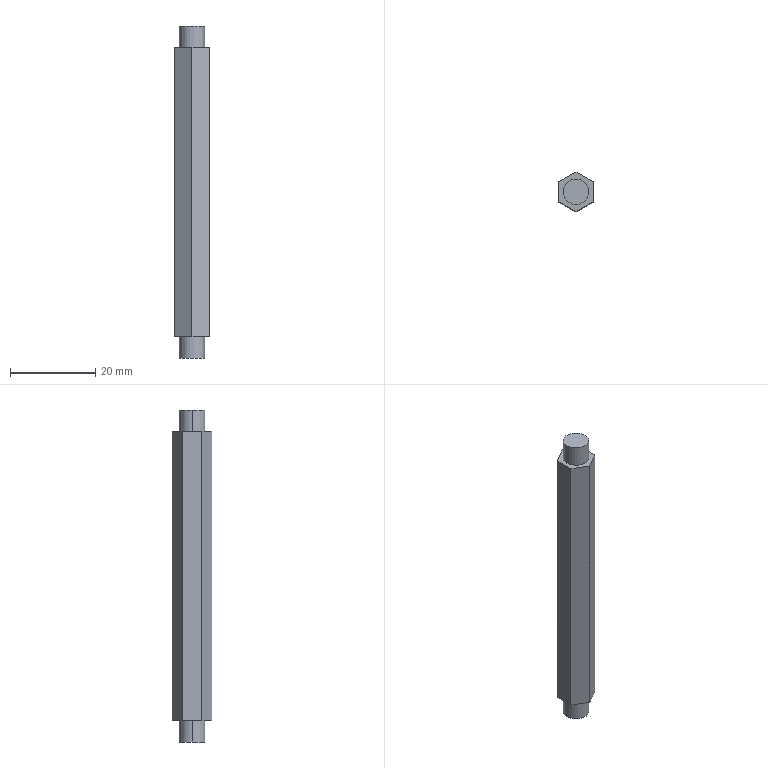Part | STEP file | 1 solid | 14 faces | box 8 x 9.238 x 78 mm | volume 4052 mm3 | plane 10 | cylinder 4 | commonest cylinder face diameters 6 x4
STEP:
#1=CARTESIAN_POINT('',(0.,0.,0.));
#2=DIRECTION('',(0.,0.,1.));
#3=DIRECTION('',(1.,0.,0.));
#4=AXIS2_PLACEMENT_3D('',#1,#2,#3);
#5=CARTESIAN_POINT('',(-5.42,-20.574,-52.535));
#6=VERTEX_POINT('',#5);
#7=CARTESIAN_POINT('',(-11.42,-20.574,-52.535));
#8=VERTEX_POINT('',#7);
#9=CARTESIAN_POINT('',(-8.42,-20.574,-52.535));
#10=DIRECTION('',(0.,0.,1.));
#11=DIRECTION('',(-1.,0.,0.));
#12=AXIS2_PLACEMENT_3D('',#9,#10,#11);
#13=CIRCLE('',#12,3.);
#14=CARTESIAN_POINT('',(-8.42,-20.574,-52.535));
#15=DIRECTION('',(0.,0.,-1.));
#16=DIRECTION('',(-1.,0.,0.));
#17=AXIS2_PLACEMENT_3D('',#14,#15,#16);
#18=CYLINDRICAL_SURFACE('',#17,3.);
#19=CARTESIAN_POINT('',(6.283,0.));
#20=DIRECTION('',(-1.,0.));
#21=VECTOR('',#20,1.);
#22=LINE('',#19,#21);
#23=(GEOMETRIC_REPRESENTATION_CONTEXT(2)PARAMETRIC_REPRESENTATION_CONTEXT()REPRESENTATION_CONTEXT('',''));
#24=DEFINITIONAL_REPRESENTATION('',(#22),#23);
#25=PCURVE('',#18,#24);
#26=CARTESIAN_POINT('',(-8.42,-20.574,-52.535));
#27=DIRECTION('',(0.,0.,-1.));
#28=DIRECTION('',(-1.,0.,0.));
#29=AXIS2_PLACEMENT_3D('',#26,#27,#28);
#30=PLANE('',#29);
#31=CARTESIAN_POINT('',(3.,0.));
#32=CARTESIAN_POINT('',(3.,-5.196));
#33=CARTESIAN_POINT('',(-1.5,-2.598));
#34=CARTESIAN_POINT('',(-6.,0.));
#35=CARTESIAN_POINT('',(-1.5,2.598));
#36=CARTESIAN_POINT('',(3.,5.196));
#37=CARTESIAN_POINT('',(3.,0.));
#38=(BOUNDED_CURVE()B_SPLINE_CURVE(2,(#31,#32,#33,#34,#35,#36,#37),.UNSPECIFIED.,.T.,.F.)B_SPLINE_CURVE_WITH_KNOTS((1,2,2,2,2,1),(-2.094,0.,2.094,4.189,6.283,8.378),.UNSPECIFIED.)CURVE()GEOMETRIC_REPRESENTATION_ITEM()RATIONAL_B_SPLINE_CURVE((1.,0.5,1.,0.5,1.,0.5,1.))REPRESENTATION_ITEM(''));
#39=(GEOMETRIC_REPRESENTATION_CONTEXT(2)PARAMETRIC_REPRESENTATION_CONTEXT()REPRESENTATION_CONTEXT('',''));
#40=DEFINITIONAL_REPRESENTATION('',(#38),#39);
#41=PCURVE('',#30,#40);
#42=SURFACE_CURVE('',#13,(#25,#41),.PCURVE_S1.);
#43=EDGE_CURVE('',#6,#8,#42,.T.);
#44=ORIENTED_EDGE('',*,*,#43,.F.);
#45=CARTESIAN_POINT('',(-5.42,-20.574,-57.535));
#46=VERTEX_POINT('',#45);
#47=CARTESIAN_POINT('',(-5.42,-20.574,-52.535));
#48=DIRECTION('',(0.,0.,-1.));
#49=VECTOR('',#48,1.);
#50=LINE('',#47,#49);
#51=CARTESIAN_POINT('',(3.142,0.));
#52=DIRECTION('',(0.,1.));
#53=VECTOR('',#52,1.);
#54=LINE('',#51,#53);
#55=(GEOMETRIC_REPRESENTATION_CONTEXT(2)PARAMETRIC_REPRESENTATION_CONTEXT()REPRESENTATION_CONTEXT('',''));
#56=DEFINITIONAL_REPRESENTATION('',(#54),#55);
#57=PCURVE('',#18,#56);
#58=CARTESIAN_POINT('',(-8.42,-20.574,-52.535));
#59=DIRECTION('',(0.,0.,-1.));
#60=DIRECTION('',(-1.,0.,0.));
#61=AXIS2_PLACEMENT_3D('',#58,#59,#60);
#62=CYLINDRICAL_SURFACE('',#61,3.);
#63=CARTESIAN_POINT('',(3.142,0.));
#64=DIRECTION('',(0.,1.));
#65=VECTOR('',#64,1.);
#66=LINE('',#63,#65);
#67=(GEOMETRIC_REPRESENTATION_CONTEXT(2)PARAMETRIC_REPRESENTATION_CONTEXT()REPRESENTATION_CONTEXT('',''));
#68=DEFINITIONAL_REPRESENTATION('',(#66),#67);
#69=PCURVE('',#62,#68);
#70=SURFACE_CURVE('',#50,(#57,#69),.PCURVE_S1.);
#71=EDGE_CURVE('',#6,#46,#70,.T.);
#72=ORIENTED_EDGE('',*,*,#71,.T.);
#73=CARTESIAN_POINT('',(-11.42,-20.574,-57.535));
#74=VERTEX_POINT('',#73);
#75=CARTESIAN_POINT('',(-8.42,-20.574,-57.535));
#76=DIRECTION('',(0.,0.,1.));
#77=DIRECTION('',(-1.,0.,0.));
#78=AXIS2_PLACEMENT_3D('',#75,#76,#77);
#79=CIRCLE('',#78,3.);
#80=CARTESIAN_POINT('',(6.283,5.));
#81=DIRECTION('',(-1.,0.));
#82=VECTOR('',#81,1.);
#83=LINE('',#80,#82);
#84=(GEOMETRIC_REPRESENTATION_CONTEXT(2)PARAMETRIC_REPRESENTATION_CONTEXT()REPRESENTATION_CONTEXT('',''));
#85=DEFINITIONAL_REPRESENTATION('',(#83),#84);
#86=PCURVE('',#18,#85);
#87=CARTESIAN_POINT('',(-8.42,-20.574,-57.535));
#88=DIRECTION('',(0.,0.,1.));
#89=DIRECTION('',(1.,0.,0.));
#90=AXIS2_PLACEMENT_3D('',#87,#88,#89);
#91=PLANE('',#90);
#92=CARTESIAN_POINT('',(0.,0.));
#93=DIRECTION('',(-1.,0.));
#94=AXIS2_PLACEMENT_2D('',#92,#93);
#95=CIRCLE('',#94,3.);
#96=(GEOMETRIC_REPRESENTATION_CONTEXT(2)PARAMETRIC_REPRESENTATION_CONTEXT()REPRESENTATION_CONTEXT('',''));
#97=DEFINITIONAL_REPRESENTATION('',(#95),#96);
#98=PCURVE('',#91,#97);
#99=SURFACE_CURVE('',#79,(#86,#98),.PCURVE_S1.);
#100=EDGE_CURVE('',#46,#74,#99,.T.);
#101=ORIENTED_EDGE('',*,*,#100,.T.);
#102=CARTESIAN_POINT('',(-11.42,-20.574,-52.535));
#103=DIRECTION('',(0.,0.,-1.));
#104=VECTOR('',#103,1.);
#105=LINE('',#102,#104);
#106=CARTESIAN_POINT('',(0.,0.));
#107=DIRECTION('',(0.,1.));
#108=VECTOR('',#107,1.);
#109=LINE('',#106,#108);
#110=(GEOMETRIC_REPRESENTATION_CONTEXT(2)PARAMETRIC_REPRESENTATION_CONTEXT()REPRESENTATION_CONTEXT('',''));
#111=DEFINITIONAL_REPRESENTATION('',(#109),#110);
#112=PCURVE('',#18,#111);
#113=CARTESIAN_POINT('',(6.283,0.));
#114=DIRECTION('',(0.,1.));
#115=VECTOR('',#114,1.);
#116=LINE('',#113,#115);
#117=(GEOMETRIC_REPRESENTATION_CONTEXT(2)PARAMETRIC_REPRESENTATION_CONTEXT()REPRESENTATION_CONTEXT('',''));
#118=DEFINITIONAL_REPRESENTATION('',(#116),#117);
#119=PCURVE('',#62,#118);
#120=SURFACE_CURVE('',#105,(#112,#119),.PCURVE_S1.);
#121=EDGE_CURVE('',#8,#74,#120,.T.);
#122=ORIENTED_EDGE('',*,*,#121,.F.);
#123=EDGE_LOOP('',(#44,#72,#101,#122));
#124=FACE_BOUND('',#123,.T.);
#125=ADVANCED_FACE('',(#124),#18,.T.);
#126=CARTESIAN_POINT('',(-11.42,-20.574,20.465));
#127=VERTEX_POINT('',#126);
#128=CARTESIAN_POINT('',(-5.42,-20.574,20.465));
#129=VERTEX_POINT('',#128);
#130=CARTESIAN_POINT('',(-8.42,-20.574,20.465));
#131=DIRECTION('',(0.,0.,-1.));
#132=DIRECTION('',(-1.,0.,0.));
#133=AXIS2_PLACEMENT_3D('',#130,#131,#132);
#134=CIRCLE('',#133,3.);
#135=CARTESIAN_POINT('',(-8.42,-20.574,15.465));
#136=DIRECTION('',(0.,0.,-1.));
#137=DIRECTION('',(-1.,0.,0.));
#138=AXIS2_PLACEMENT_3D('',#135,#136,#137);
#139=CYLINDRICAL_SURFACE('',#138,3.);
#140=CARTESIAN_POINT('',(0.,-5.));
#141=DIRECTION('',(1.,0.));
#142=VECTOR('',#141,1.);
#143=LINE('',#140,#142);
#144=(GEOMETRIC_REPRESENTATION_CONTEXT(2)PARAMETRIC_REPRESENTATION_CONTEXT()REPRESENTATION_CONTEXT('',''));
#145=DEFINITIONAL_REPRESENTATION('',(#143),#144);
#146=PCURVE('',#139,#145);
#147=CARTESIAN_POINT('',(-8.42,-20.574,20.465));
#148=DIRECTION('',(0.,0.,1.));
#149=DIRECTION('',(1.,0.,0.));
#150=AXIS2_PLACEMENT_3D('',#147,#148,#149);
#151=PLANE('',#150);
#152=CARTESIAN_POINT('',(-3.,0.));
#153=CARTESIAN_POINT('',(-3.,5.196));
#154=CARTESIAN_POINT('',(1.5,2.598));
#155=CARTESIAN_POINT('',(6.,0.));
#156=CARTESIAN_POINT('',(1.5,-2.598));
#157=CARTESIAN_POINT('',(-3.,-5.196));
#158=CARTESIAN_POINT('',(-3.,0.));
#159=(BOUNDED_CURVE()B_SPLINE_CURVE(2,(#152,#153,#154,#155,#156,#157,#158),.UNSPECIFIED.,.T.,.F.)B_SPLINE_CURVE_WITH_KNOTS((1,2,2,2,2,1),(-2.094,0.,2.094,4.189,6.283,8.378),.UNSPECIFIED.)CURVE()GEOMETRIC_REPRESENTATION_ITEM()RATIONAL_B_SPLINE_CURVE((1.,0.5,1.,0.5,1.,0.5,1.))REPRESENTATION_ITEM(''));
#160=(GEOMETRIC_REPRESENTATION_CONTEXT(2)PARAMETRIC_REPRESENTATION_CONTEXT()REPRESENTATION_CONTEXT('',''));
#161=DEFINITIONAL_REPRESENTATION('',(#159),#160);
#162=PCURVE('',#151,#161);
#163=SURFACE_CURVE('',#134,(#146,#162),.PCURVE_S1.);
#164=EDGE_CURVE('',#127,#129,#163,.T.);
#165=ORIENTED_EDGE('',*,*,#164,.T.);
#166=CARTESIAN_POINT('',(-5.42,-20.574,15.465));
#167=VERTEX_POINT('',#166);
#168=CARTESIAN_POINT('',(-5.42,-20.574,15.465));
#169=DIRECTION('',(0.,0.,-1.));
#170=VECTOR('',#169,1.);
#171=LINE('',#168,#170);
#172=CARTESIAN_POINT('',(3.142,0.));
#173=DIRECTION('',(0.,1.));
#174=VECTOR('',#173,1.);
#175=LINE('',#172,#174);
#176=(GEOMETRIC_REPRESENTATION_CONTEXT(2)PARAMETRIC_REPRESENTATION_CONTEXT()REPRESENTATION_CONTEXT('',''));
#177=DEFINITIONAL_REPRESENTATION('',(#175),#176);
#178=PCURVE('',#139,#177);
#179=CARTESIAN_POINT('',(-8.42,-20.574,15.465));
#180=DIRECTION('',(0.,0.,-1.));
#181=DIRECTION('',(-1.,0.,0.));
#182=AXIS2_PLACEMENT_3D('',#179,#180,#181);
#183=CYLINDRICAL_SURFACE('',#182,3.);
#184=CARTESIAN_POINT('',(3.142,0.));
#185=DIRECTION('',(0.,1.));
#186=VECTOR('',#185,1.);
#187=LINE('',#184,#186);
#188=(GEOMETRIC_REPRESENTATION_CONTEXT(2)PARAMETRIC_REPRESENTATION_CONTEXT()REPRESENTATION_CONTEXT('',''));
#189=DEFINITIONAL_REPRESENTATION('',(#187),#188);
#190=PCURVE('',#183,#189);
#191=SURFACE_CURVE('',#171,(#178,#190),.PCURVE_S1.);
#192=EDGE_CURVE('',#129,#167,#191,.T.);
#193=ORIENTED_EDGE('',*,*,#192,.T.);
#194=CARTESIAN_POINT('',(-11.42,-20.574,15.465));
#195=VERTEX_POINT('',#194);
#196=CARTESIAN_POINT('',(-8.42,-20.574,15.465));
#197=DIRECTION('',(0.,0.,-1.));
#198=DIRECTION('',(-1.,0.,0.));
#199=AXIS2_PLACEMENT_3D('',#196,#197,#198);
#200=CIRCLE('',#199,3.);
#201=CARTESIAN_POINT('',(0.,0.));
#202=DIRECTION('',(1.,0.));
#203=VECTOR('',#202,1.);
#204=LINE('',#201,#203);
#205=(GEOMETRIC_REPRESENTATION_CONTEXT(2)PARAMETRIC_REPRESENTATION_CONTEXT()REPRESENTATION_CONTEXT('',''));
#206=DEFINITIONAL_REPRESENTATION('',(#204),#205);
#207=PCURVE('',#139,#206);
#208=CARTESIAN_POINT('',(-8.42,-20.574,15.465));
#209=DIRECTION('',(0.,0.,1.));
#210=DIRECTION('',(1.,0.,0.));
#211=AXIS2_PLACEMENT_3D('',#208,#209,#210);
#212=PLANE('',#211);
#213=CARTESIAN_POINT('',(-3.,0.));
#214=CARTESIAN_POINT('',(-3.,5.196));
#215=CARTESIAN_POINT('',(1.5,2.598));
#216=CARTESIAN_POINT('',(6.,0.));
#217=CARTESIAN_POINT('',(1.5,-2.598));
#218=CARTESIAN_POINT('',(-3.,-5.196));
#219=CARTESIAN_POINT('',(-3.,0.));
#220=(BOUNDED_CURVE()B_SPLINE_CURVE(2,(#213,#214,#215,#216,#217,#218,#219),.UNSPECIFIED.,.T.,.F.)B_SPLINE_CURVE_WITH_KNOTS((1,2,2,2,2,1),(-2.094,0.,2.094,4.189,6.283,8.378),.UNSPECIFIED.)CURVE()GEOMETRIC_REPRESENTATION_ITEM()RATIONAL_B_SPLINE_CURVE((1.,0.5,1.,0.5,1.,0.5,1.))REPRESENTATION_ITEM(''));
#221=(GEOMETRIC_REPRESENTATION_CONTEXT(2)PARAMETRIC_REPRESENTATION_CONTEXT()REPRESENTATION_CONTEXT('',''));
#222=DEFINITIONAL_REPRESENTATION('',(#220),#221);
#223=PCURVE('',#212,#222);
#224=SURFACE_CURVE('',#200,(#207,#223),.PCURVE_S1.);
#225=EDGE_CURVE('',#195,#167,#224,.T.);
#226=ORIENTED_EDGE('',*,*,#225,.F.);
#227=CARTESIAN_POINT('',(-11.42,-20.574,15.465));
#228=DIRECTION('',(0.,0.,-1.));
#229=VECTOR('',#228,1.);
#230=LINE('',#227,#229);
#231=CARTESIAN_POINT('',(0.,0.));
#232=DIRECTION('',(0.,1.));
#233=VECTOR('',#232,1.);
#234=LINE('',#231,#233);
#235=(GEOMETRIC_REPRESENTATION_CONTEXT(2)PARAMETRIC_REPRESENTATION_CONTEXT()REPRESENTATION_CONTEXT('',''));
#236=DEFINITIONAL_REPRESENTATION('',(#234),#235);
#237=PCURVE('',#139,#236);
#238=CARTESIAN_POINT('',(6.283,0.));
#239=DIRECTION('',(0.,1.));
#240=VECTOR('',#239,1.);
#241=LINE('',#238,#240);
#242=(GEOMETRIC_REPRESENTATION_CONTEXT(2)PARAMETRIC_REPRESENTATION_CONTEXT()REPRESENTATION_CONTEXT('',''));
#243=DEFINITIONAL_REPRESENTATION('',(#241),#242);
#244=PCURVE('',#183,#243);
#245=SURFACE_CURVE('',#230,(#237,#244),.PCURVE_S1.);
#246=EDGE_CURVE('',#127,#195,#245,.T.);
#247=ORIENTED_EDGE('',*,*,#246,.F.);
#248=EDGE_LOOP('',(#165,#193,#226,#247));
#249=FACE_BOUND('',#248,.T.);
#250=ADVANCED_FACE('',(#249),#139,.T.);
#251=CARTESIAN_POINT('',(-8.42,-25.193,15.465));
#252=VERTEX_POINT('',#251);
#253=CARTESIAN_POINT('',(-8.42,-25.193,-52.535));
#254=VERTEX_POINT('',#253);
#255=CARTESIAN_POINT('',(-8.42,-25.193,-18.535));
#256=DIRECTION('',(0.,0.,-1.));
#257=VECTOR('',#256,1.);
#258=LINE('',#255,#257);
#259=CARTESIAN_POINT('',(-8.42,-25.193,-18.535));
#260=DIRECTION('',(0.5,-0.866,0.));
#261=DIRECTION('',(0.866,0.5,0.));
#262=AXIS2_PLACEMENT_3D('',#259,#260,#261);
#263=PLANE('',#262);
#264=CARTESIAN_POINT('',(0.,0.));
#265=DIRECTION('',(0.,-1.));
#266=VECTOR('',#265,1.);
#267=LINE('',#264,#266);
#268=(GEOMETRIC_REPRESENTATION_CONTEXT(2)PARAMETRIC_REPRESENTATION_CONTEXT()REPRESENTATION_CONTEXT('',''));
#269=DEFINITIONAL_REPRESENTATION('',(#267),#268);
#270=PCURVE('',#263,#269);
#271=CARTESIAN_POINT('',(-12.42,-22.883,-18.535));
#272=DIRECTION('',(-0.5,-0.866,0.));
#273=DIRECTION('',(0.866,-0.5,0.));
#274=AXIS2_PLACEMENT_3D('',#271,#272,#273);
#275=PLANE('',#274);
#276=CARTESIAN_POINT('',(4.619,0.));
#277=DIRECTION('',(0.,-1.));
#278=VECTOR('',#277,1.);
#279=LINE('',#276,#278);
#280=(GEOMETRIC_REPRESENTATION_CONTEXT(2)PARAMETRIC_REPRESENTATION_CONTEXT()REPRESENTATION_CONTEXT('',''));
#281=DEFINITIONAL_REPRESENTATION('',(#279),#280);
#282=PCURVE('',#275,#281);
#283=SURFACE_CURVE('',#258,(#270,#282),.PCURVE_S1.);
#284=EDGE_CURVE('',#252,#254,#283,.T.);
#285=ORIENTED_EDGE('',*,*,#284,.T.);
#286=CARTESIAN_POINT('',(-4.42,-22.883,-52.535));
#287=VERTEX_POINT('',#286);
#288=CARTESIAN_POINT('',(-8.42,-25.193,-52.535));
#289=DIRECTION('',(0.866,0.5,0.));
#290=VECTOR('',#289,1.);
#291=LINE('',#288,#290);
#292=CARTESIAN_POINT('',(0.,-34.));
#293=DIRECTION('',(1.,0.));
#294=VECTOR('',#293,1.);
#295=LINE('',#292,#294);
#296=(GEOMETRIC_REPRESENTATION_CONTEXT(2)PARAMETRIC_REPRESENTATION_CONTEXT()REPRESENTATION_CONTEXT('',''));
#297=DEFINITIONAL_REPRESENTATION('',(#295),#296);
#298=PCURVE('',#263,#297);
#299=CARTESIAN_POINT('',(0.,-4.619));
#300=DIRECTION('',(-0.866,0.5));
#301=VECTOR('',#300,1.);
#302=LINE('',#299,#301);
#303=(GEOMETRIC_REPRESENTATION_CONTEXT(2)PARAMETRIC_REPRESENTATION_CONTEXT()REPRESENTATION_CONTEXT('',''));
#304=DEFINITIONAL_REPRESENTATION('',(#302),#303);
#305=PCURVE('',#30,#304);
#306=SURFACE_CURVE('',#291,(#298,#305),.PCURVE_S1.);
#307=EDGE_CURVE('',#254,#287,#306,.T.);
#308=ORIENTED_EDGE('',*,*,#307,.T.);
#309=CARTESIAN_POINT('',(-4.42,-22.883,15.465));
#310=VERTEX_POINT('',#309);
#311=CARTESIAN_POINT('',(-4.42,-22.883,-18.535));
#312=DIRECTION('',(0.,0.,1.));
#313=VECTOR('',#312,1.);
#314=LINE('',#311,#313);
#315=CARTESIAN_POINT('',(4.619,0.));
#316=DIRECTION('',(0.,1.));
#317=VECTOR('',#316,1.);
#318=LINE('',#315,#317);
#319=(GEOMETRIC_REPRESENTATION_CONTEXT(2)PARAMETRIC_REPRESENTATION_CONTEXT()REPRESENTATION_CONTEXT('',''));
#320=DEFINITIONAL_REPRESENTATION('',(#318),#319);
#321=PCURVE('',#263,#320);
#322=CARTESIAN_POINT('',(-4.42,-22.883,-18.535));
#323=DIRECTION('',(1.,0.,0.));
#324=DIRECTION('',(0.,1.,0.));
#325=AXIS2_PLACEMENT_3D('',#322,#323,#324);
#326=PLANE('',#325);
#327=CARTESIAN_POINT('',(0.,0.));
#328=DIRECTION('',(0.,1.));
#329=VECTOR('',#328,1.);
#330=LINE('',#327,#329);
#331=(GEOMETRIC_REPRESENTATION_CONTEXT(2)PARAMETRIC_REPRESENTATION_CONTEXT()REPRESENTATION_CONTEXT('',''));
#332=DEFINITIONAL_REPRESENTATION('',(#330),#331);
#333=PCURVE('',#326,#332);
#334=SURFACE_CURVE('',#314,(#321,#333),.PCURVE_S1.);
#335=EDGE_CURVE('',#287,#310,#334,.T.);
#336=ORIENTED_EDGE('',*,*,#335,.T.);
#337=CARTESIAN_POINT('',(-8.42,-25.193,15.465));
#338=DIRECTION('',(-0.866,-0.5,0.));
#339=VECTOR('',#338,1.);
#340=LINE('',#337,#339);
#341=CARTESIAN_POINT('',(0.,34.));
#342=DIRECTION('',(-1.,0.));
#343=VECTOR('',#342,1.);
#344=LINE('',#341,#343);
#345=(GEOMETRIC_REPRESENTATION_CONTEXT(2)PARAMETRIC_REPRESENTATION_CONTEXT()REPRESENTATION_CONTEXT('',''));
#346=DEFINITIONAL_REPRESENTATION('',(#344),#345);
#347=PCURVE('',#263,#346);
#348=CARTESIAN_POINT('',(0.,-4.619));
#349=DIRECTION('',(-0.866,-0.5));
#350=VECTOR('',#349,1.);
#351=LINE('',#348,#350);
#352=(GEOMETRIC_REPRESENTATION_CONTEXT(2)PARAMETRIC_REPRESENTATION_CONTEXT()REPRESENTATION_CONTEXT('',''));
#353=DEFINITIONAL_REPRESENTATION('',(#351),#352);
#354=PCURVE('',#212,#353);
#355=SURFACE_CURVE('',#340,(#347,#354),.PCURVE_S1.);
#356=EDGE_CURVE('',#310,#252,#355,.T.);
#357=ORIENTED_EDGE('',*,*,#356,.T.);
#358=EDGE_LOOP('',(#285,#308,#336,#357));
#359=FACE_BOUND('',#358,.T.);
#360=ADVANCED_FACE('',(#359),#263,.T.);
#361=CARTESIAN_POINT('',(-12.42,-22.883,-52.535));
#362=VERTEX_POINT('',#361);
#363=CARTESIAN_POINT('',(-8.42,-25.193,-52.535));
#364=DIRECTION('',(-0.866,0.5,0.));
#365=VECTOR('',#364,1.);
#366=LINE('',#363,#365);
#367=CARTESIAN_POINT('',(0.,-4.619));
#368=DIRECTION('',(0.866,0.5));
#369=VECTOR('',#368,1.);
#370=LINE('',#367,#369);
#371=(GEOMETRIC_REPRESENTATION_CONTEXT(2)PARAMETRIC_REPRESENTATION_CONTEXT()REPRESENTATION_CONTEXT('',''));
#372=DEFINITIONAL_REPRESENTATION('',(#370),#371);
#373=PCURVE('',#30,#372);
#374=CARTESIAN_POINT('',(4.619,-34.));
#375=DIRECTION('',(-1.,0.));
#376=VECTOR('',#375,1.);
#377=LINE('',#374,#376);
#378=(GEOMETRIC_REPRESENTATION_CONTEXT(2)PARAMETRIC_REPRESENTATION_CONTEXT()REPRESENTATION_CONTEXT('',''));
#379=DEFINITIONAL_REPRESENTATION('',(#377),#378);
#380=PCURVE('',#275,#379);
#381=SURFACE_CURVE('',#366,(#373,#380),.PCURVE_S1.);
#382=EDGE_CURVE('',#254,#362,#381,.T.);
#383=ORIENTED_EDGE('',*,*,#382,.T.);
#384=CARTESIAN_POINT('',(-12.42,-18.264,-52.535));
#385=VERTEX_POINT('',#384);
#386=CARTESIAN_POINT('',(-12.42,-20.574,-52.535));
#387=DIRECTION('',(0.,1.,0.));
#388=VECTOR('',#387,1.);
#389=LINE('',#386,#388);
#390=CARTESIAN_POINT('',(4.,0.));
#391=DIRECTION('',(0.,1.));
#392=VECTOR('',#391,1.);
#393=LINE('',#390,#392);
#394=(GEOMETRIC_REPRESENTATION_CONTEXT(2)PARAMETRIC_REPRESENTATION_CONTEXT()REPRESENTATION_CONTEXT('',''));
#395=DEFINITIONAL_REPRESENTATION('',(#393),#394);
#396=PCURVE('',#30,#395);
#397=CARTESIAN_POINT('',(-12.42,-18.264,-18.535));
#398=DIRECTION('',(-1.,0.,0.));
#399=DIRECTION('',(0.,-1.,0.));
#400=AXIS2_PLACEMENT_3D('',#397,#398,#399);
#401=PLANE('',#400);
#402=CARTESIAN_POINT('',(2.309,-34.));
#403=DIRECTION('',(-1.,0.));
#404=VECTOR('',#403,1.);
#405=LINE('',#402,#404);
#406=(GEOMETRIC_REPRESENTATION_CONTEXT(2)PARAMETRIC_REPRESENTATION_CONTEXT()REPRESENTATION_CONTEXT('',''));
#407=DEFINITIONAL_REPRESENTATION('',(#405),#406);
#408=PCURVE('',#401,#407);
#409=SURFACE_CURVE('',#389,(#396,#408),.PCURVE_S1.);
#410=EDGE_CURVE('',#362,#385,#409,.T.);
#411=ORIENTED_EDGE('',*,*,#410,.T.);
#412=CARTESIAN_POINT('',(-8.42,-15.955,-52.535));
#413=VERTEX_POINT('',#412);
#414=CARTESIAN_POINT('',(-12.42,-18.264,-52.535));
#415=DIRECTION('',(0.866,0.5,0.));
#416=VECTOR('',#415,1.);
#417=LINE('',#414,#416);
#418=CARTESIAN_POINT('',(4.,2.309));
#419=DIRECTION('',(-0.866,0.5));
#420=VECTOR('',#419,1.);
#421=LINE('',#418,#420);
#422=(GEOMETRIC_REPRESENTATION_CONTEXT(2)PARAMETRIC_REPRESENTATION_CONTEXT()REPRESENTATION_CONTEXT('',''));
#423=DEFINITIONAL_REPRESENTATION('',(#421),#422);
#424=PCURVE('',#30,#423);
#425=CARTESIAN_POINT('',(-8.42,-15.955,-18.535));
#426=DIRECTION('',(-0.5,0.866,0.));
#427=DIRECTION('',(-0.866,-0.5,0.));
#428=AXIS2_PLACEMENT_3D('',#425,#426,#427);
#429=PLANE('',#428);
#430=CARTESIAN_POINT('',(4.619,-34.));
#431=DIRECTION('',(-1.,0.));
#432=VECTOR('',#431,1.);
#433=LINE('',#430,#432);
#434=(GEOMETRIC_REPRESENTATION_CONTEXT(2)PARAMETRIC_REPRESENTATION_CONTEXT()REPRESENTATION_CONTEXT('',''));
#435=DEFINITIONAL_REPRESENTATION('',(#433),#434);
#436=PCURVE('',#429,#435);
#437=SURFACE_CURVE('',#417,(#424,#436),.PCURVE_S1.);
#438=EDGE_CURVE('',#385,#413,#437,.T.);
#439=ORIENTED_EDGE('',*,*,#438,.T.);
#440=CARTESIAN_POINT('',(-4.42,-18.264,-52.535));
#441=VERTEX_POINT('',#440);
#442=CARTESIAN_POINT('',(-8.42,-15.955,-52.535));
#443=DIRECTION('',(0.866,-0.5,0.));
#444=VECTOR('',#443,1.);
#445=LINE('',#442,#444);
#446=CARTESIAN_POINT('',(0.,4.619));
#447=DIRECTION('',(-0.866,-0.5));
#448=VECTOR('',#447,1.);
#449=LINE('',#446,#448);
#450=(GEOMETRIC_REPRESENTATION_CONTEXT(2)PARAMETRIC_REPRESENTATION_CONTEXT()REPRESENTATION_CONTEXT('',''));
#451=DEFINITIONAL_REPRESENTATION('',(#449),#450);
#452=PCURVE('',#30,#451);
#453=CARTESIAN_POINT('',(-4.42,-18.264,-18.535));
#454=DIRECTION('',(0.5,0.866,0.));
#455=DIRECTION('',(-0.866,0.5,0.));
#456=AXIS2_PLACEMENT_3D('',#453,#454,#455);
#457=PLANE('',#456);
#458=CARTESIAN_POINT('',(4.619,-34.));
#459=DIRECTION('',(-1.,0.));
#460=VECTOR('',#459,1.);
#461=LINE('',#458,#460);
#462=(GEOMETRIC_REPRESENTATION_CONTEXT(2)PARAMETRIC_REPRESENTATION_CONTEXT()REPRESENTATION_CONTEXT('',''));
#463=DEFINITIONAL_REPRESENTATION('',(#461),#462);
#464=PCURVE('',#457,#463);
#465=SURFACE_CURVE('',#445,(#452,#464),.PCURVE_S1.);
#466=EDGE_CURVE('',#413,#441,#465,.T.);
#467=ORIENTED_EDGE('',*,*,#466,.T.);
#468=CARTESIAN_POINT('',(-4.42,-20.574,-52.535));
#469=DIRECTION('',(0.,-1.,0.));
#470=VECTOR('',#469,1.);
#471=LINE('',#468,#470);
#472=CARTESIAN_POINT('',(-4.,0.));
#473=DIRECTION('',(0.,-1.));
#474=VECTOR('',#473,1.);
#475=LINE('',#472,#474);
#476=(GEOMETRIC_REPRESENTATION_CONTEXT(2)PARAMETRIC_REPRESENTATION_CONTEXT()REPRESENTATION_CONTEXT('',''));
#477=DEFINITIONAL_REPRESENTATION('',(#475),#476);
#478=PCURVE('',#30,#477);
#479=CARTESIAN_POINT('',(2.309,-34.));
#480=DIRECTION('',(-1.,0.));
#481=VECTOR('',#480,1.);
#482=LINE('',#479,#481);
#483=(GEOMETRIC_REPRESENTATION_CONTEXT(2)PARAMETRIC_REPRESENTATION_CONTEXT()REPRESENTATION_CONTEXT('',''));
#484=DEFINITIONAL_REPRESENTATION('',(#482),#483);
#485=PCURVE('',#326,#484);
#486=SURFACE_CURVE('',#471,(#478,#485),.PCURVE_S1.);
#487=EDGE_CURVE('',#441,#287,#486,.T.);
#488=ORIENTED_EDGE('',*,*,#487,.T.);
#489=ORIENTED_EDGE('',*,*,#307,.F.);
#490=EDGE_LOOP('',(#383,#411,#439,#467,#488,#489));
#491=FACE_BOUND('',#490,.T.);
#492=CARTESIAN_POINT('',(-8.42,-20.574,-52.535));
#493=DIRECTION('',(0.,0.,1.));
#494=DIRECTION('',(-1.,0.,0.));
#495=AXIS2_PLACEMENT_3D('',#492,#493,#494);
#496=CIRCLE('',#495,3.);
#497=CARTESIAN_POINT('',(3.,0.));
#498=CARTESIAN_POINT('',(3.,-5.196));
#499=CARTESIAN_POINT('',(-1.5,-2.598));
#500=CARTESIAN_POINT('',(-6.,0.));
#501=CARTESIAN_POINT('',(-1.5,2.598));
#502=CARTESIAN_POINT('',(3.,5.196));
#503=CARTESIAN_POINT('',(3.,0.));
#504=(BOUNDED_CURVE()B_SPLINE_CURVE(2,(#497,#498,#499,#500,#501,#502,#503),.UNSPECIFIED.,.T.,.F.)B_SPLINE_CURVE_WITH_KNOTS((1,2,2,2,2,1),(-2.094,0.,2.094,4.189,6.283,8.378),.UNSPECIFIED.)CURVE()GEOMETRIC_REPRESENTATION_ITEM()RATIONAL_B_SPLINE_CURVE((1.,0.5,1.,0.5,1.,0.5,1.))REPRESENTATION_ITEM(''));
#505=(GEOMETRIC_REPRESENTATION_CONTEXT(2)PARAMETRIC_REPRESENTATION_CONTEXT()REPRESENTATION_CONTEXT('',''));
#506=DEFINITIONAL_REPRESENTATION('',(#504),#505);
#507=PCURVE('',#30,#506);
#508=CARTESIAN_POINT('',(6.283,0.));
#509=DIRECTION('',(-1.,0.));
#510=VECTOR('',#509,1.);
#511=LINE('',#508,#510);
#512=(GEOMETRIC_REPRESENTATION_CONTEXT(2)PARAMETRIC_REPRESENTATION_CONTEXT()REPRESENTATION_CONTEXT('',''));
#513=DEFINITIONAL_REPRESENTATION('',(#511),#512);
#514=PCURVE('',#62,#513);
#515=SURFACE_CURVE('',#496,(#507,#514),.PCURVE_S1.);
#516=EDGE_CURVE('',#8,#6,#515,.T.);
#517=ORIENTED_EDGE('',*,*,#516,.T.);
#518=ORIENTED_EDGE('',*,*,#43,.T.);
#519=EDGE_LOOP('',(#517,#518));
#520=FACE_BOUND('',#519,.T.);
#521=ADVANCED_FACE('',(#491,#520),#30,.T.);
#522=CARTESIAN_POINT('',(-12.42,-22.883,15.465));
#523=VERTEX_POINT('',#522);
#524=CARTESIAN_POINT('',(-12.42,-22.883,-18.535));
#525=DIRECTION('',(0.,0.,-1.));
#526=VECTOR('',#525,1.);
#527=LINE('',#524,#526);
#528=CARTESIAN_POINT('',(0.,0.));
#529=DIRECTION('',(0.,-1.));
#530=VECTOR('',#529,1.);
#531=LINE('',#528,#530);
#532=(GEOMETRIC_REPRESENTATION_CONTEXT(2)PARAMETRIC_REPRESENTATION_CONTEXT()REPRESENTATION_CONTEXT('',''));
#533=DEFINITIONAL_REPRESENTATION('',(#531),#532);
#534=PCURVE('',#275,#533);
#535=CARTESIAN_POINT('',(4.619,0.));
#536=DIRECTION('',(0.,-1.));
#537=VECTOR('',#536,1.);
#538=LINE('',#535,#537);
#539=(GEOMETRIC_REPRESENTATION_CONTEXT(2)PARAMETRIC_REPRESENTATION_CONTEXT()REPRESENTATION_CONTEXT('',''));
#540=DEFINITIONAL_REPRESENTATION('',(#538),#539);
#541=PCURVE('',#401,#540);
#542=SURFACE_CURVE('',#527,(#534,#541),.PCURVE_S1.);
#543=EDGE_CURVE('',#523,#362,#542,.T.);
#544=ORIENTED_EDGE('',*,*,#543,.T.);
#545=ORIENTED_EDGE('',*,*,#382,.F.);
#546=ORIENTED_EDGE('',*,*,#284,.F.);
#547=CARTESIAN_POINT('',(-12.42,-22.883,15.465));
#548=DIRECTION('',(-0.866,0.5,0.));
#549=VECTOR('',#548,1.);
#550=LINE('',#547,#549);
#551=CARTESIAN_POINT('',(0.,34.));
#552=DIRECTION('',(-1.,0.));
#553=VECTOR('',#552,1.);
#554=LINE('',#551,#553);
#555=(GEOMETRIC_REPRESENTATION_CONTEXT(2)PARAMETRIC_REPRESENTATION_CONTEXT()REPRESENTATION_CONTEXT('',''));
#556=DEFINITIONAL_REPRESENTATION('',(#554),#555);
#557=PCURVE('',#275,#556);
#558=CARTESIAN_POINT('',(-4.,-2.309));
#559=DIRECTION('',(-0.866,0.5));
#560=VECTOR('',#559,1.);
#561=LINE('',#558,#560);
#562=(GEOMETRIC_REPRESENTATION_CONTEXT(2)PARAMETRIC_REPRESENTATION_CONTEXT()REPRESENTATION_CONTEXT('',''));
#563=DEFINITIONAL_REPRESENTATION('',(#561),#562);
#564=PCURVE('',#212,#563);
#565=SURFACE_CURVE('',#550,(#557,#564),.PCURVE_S1.);
#566=EDGE_CURVE('',#252,#523,#565,.T.);
#567=ORIENTED_EDGE('',*,*,#566,.T.);
#568=EDGE_LOOP('',(#544,#545,#546,#567));
#569=FACE_BOUND('',#568,.T.);
#570=ADVANCED_FACE('',(#569),#275,.T.);
#571=CARTESIAN_POINT('',(-4.42,-18.264,15.465));
#572=VERTEX_POINT('',#571);
#573=CARTESIAN_POINT('',(-4.42,-20.574,15.465));
#574=DIRECTION('',(0.,1.,0.));
#575=VECTOR('',#574,1.);
#576=LINE('',#573,#575);
#577=CARTESIAN_POINT('',(4.,0.));
#578=DIRECTION('',(0.,1.));
#579=VECTOR('',#578,1.);
#580=LINE('',#577,#579);
#581=(GEOMETRIC_REPRESENTATION_CONTEXT(2)PARAMETRIC_REPRESENTATION_CONTEXT()REPRESENTATION_CONTEXT('',''));
#582=DEFINITIONAL_REPRESENTATION('',(#580),#581);
#583=PCURVE('',#212,#582);
#584=CARTESIAN_POINT('',(2.309,34.));
#585=DIRECTION('',(1.,0.));
#586=VECTOR('',#585,1.);
#587=LINE('',#584,#586);
#588=(GEOMETRIC_REPRESENTATION_CONTEXT(2)PARAMETRIC_REPRESENTATION_CONTEXT()REPRESENTATION_CONTEXT('',''));
#589=DEFINITIONAL_REPRESENTATION('',(#587),#588);
#590=PCURVE('',#326,#589);
#591=SURFACE_CURVE('',#576,(#583,#590),.PCURVE_S1.);
#592=EDGE_CURVE('',#310,#572,#591,.T.);
#593=ORIENTED_EDGE('',*,*,#592,.T.);
#594=CARTESIAN_POINT('',(-8.42,-15.955,15.465));
#595=VERTEX_POINT('',#594);
#596=CARTESIAN_POINT('',(-4.42,-18.264,15.465));
#597=DIRECTION('',(-0.866,0.5,0.));
#598=VECTOR('',#597,1.);
#599=LINE('',#596,#598);
#600=CARTESIAN_POINT('',(4.,2.309));
#601=DIRECTION('',(-0.866,0.5));
#602=VECTOR('',#601,1.);
#603=LINE('',#600,#602);
#604=(GEOMETRIC_REPRESENTATION_CONTEXT(2)PARAMETRIC_REPRESENTATION_CONTEXT()REPRESENTATION_CONTEXT('',''));
#605=DEFINITIONAL_REPRESENTATION('',(#603),#604);
#606=PCURVE('',#212,#605);
#607=CARTESIAN_POINT('',(0.,34.));
#608=DIRECTION('',(1.,0.));
#609=VECTOR('',#608,1.);
#610=LINE('',#607,#609);
#611=(GEOMETRIC_REPRESENTATION_CONTEXT(2)PARAMETRIC_REPRESENTATION_CONTEXT()REPRESENTATION_CONTEXT('',''));
#612=DEFINITIONAL_REPRESENTATION('',(#610),#611);
#613=PCURVE('',#457,#612);
#614=SURFACE_CURVE('',#599,(#606,#613),.PCURVE_S1.);
#615=EDGE_CURVE('',#572,#595,#614,.T.);
#616=ORIENTED_EDGE('',*,*,#615,.T.);
#617=CARTESIAN_POINT('',(-12.42,-18.264,15.465));
#618=VERTEX_POINT('',#617);
#619=CARTESIAN_POINT('',(-8.42,-15.955,15.465));
#620=DIRECTION('',(-0.866,-0.5,0.));
#621=VECTOR('',#620,1.);
#622=LINE('',#619,#621);
#623=CARTESIAN_POINT('',(0.,4.619));
#624=DIRECTION('',(-0.866,-0.5));
#625=VECTOR('',#624,1.);
#626=LINE('',#623,#625);
#627=(GEOMETRIC_REPRESENTATION_CONTEXT(2)PARAMETRIC_REPRESENTATION_CONTEXT()REPRESENTATION_CONTEXT('',''));
#628=DEFINITIONAL_REPRESENTATION('',(#626),#627);
#629=PCURVE('',#212,#628);
#630=CARTESIAN_POINT('',(0.,34.));
#631=DIRECTION('',(1.,0.));
#632=VECTOR('',#631,1.);
#633=LINE('',#630,#632);
#634=(GEOMETRIC_REPRESENTATION_CONTEXT(2)PARAMETRIC_REPRESENTATION_CONTEXT()REPRESENTATION_CONTEXT('',''));
#635=DEFINITIONAL_REPRESENTATION('',(#633),#634);
#636=PCURVE('',#429,#635);
#637=SURFACE_CURVE('',#622,(#629,#636),.PCURVE_S1.);
#638=EDGE_CURVE('',#595,#618,#637,.T.);
#639=ORIENTED_EDGE('',*,*,#638,.T.);
#640=CARTESIAN_POINT('',(-12.42,-20.574,15.465));
#641=DIRECTION('',(0.,-1.,0.));
#642=VECTOR('',#641,1.);
#643=LINE('',#640,#642);
#644=CARTESIAN_POINT('',(-4.,0.));
#645=DIRECTION('',(0.,-1.));
#646=VECTOR('',#645,1.);
#647=LINE('',#644,#646);
#648=(GEOMETRIC_REPRESENTATION_CONTEXT(2)PARAMETRIC_REPRESENTATION_CONTEXT()REPRESENTATION_CONTEXT('',''));
#649=DEFINITIONAL_REPRESENTATION('',(#647),#648);
#650=PCURVE('',#212,#649);
#651=CARTESIAN_POINT('',(2.309,34.));
#652=DIRECTION('',(1.,0.));
#653=VECTOR('',#652,1.);
#654=LINE('',#651,#653);
#655=(GEOMETRIC_REPRESENTATION_CONTEXT(2)PARAMETRIC_REPRESENTATION_CONTEXT()REPRESENTATION_CONTEXT('',''));
#656=DEFINITIONAL_REPRESENTATION('',(#654),#655);
#657=PCURVE('',#401,#656);
#658=SURFACE_CURVE('',#643,(#650,#657),.PCURVE_S1.);
#659=EDGE_CURVE('',#618,#523,#658,.T.);
#660=ORIENTED_EDGE('',*,*,#659,.T.);
#661=ORIENTED_EDGE('',*,*,#566,.F.);
#662=ORIENTED_EDGE('',*,*,#356,.F.);
#663=EDGE_LOOP('',(#593,#616,#639,#660,#661,#662));
#664=FACE_BOUND('',#663,.T.);
#665=ORIENTED_EDGE('',*,*,#225,.T.);
#666=CARTESIAN_POINT('',(-8.42,-20.574,15.465));
#667=DIRECTION('',(0.,0.,-1.));
#668=DIRECTION('',(-1.,0.,0.));
#669=AXIS2_PLACEMENT_3D('',#666,#667,#668);
#670=CIRCLE('',#669,3.);
#671=CARTESIAN_POINT('',(-3.,0.));
#672=CARTESIAN_POINT('',(-3.,5.196));
#673=CARTESIAN_POINT('',(1.5,2.598));
#674=CARTESIAN_POINT('',(6.,0.));
#675=CARTESIAN_POINT('',(1.5,-2.598));
#676=CARTESIAN_POINT('',(-3.,-5.196));
#677=CARTESIAN_POINT('',(-3.,0.));
#678=(BOUNDED_CURVE()B_SPLINE_CURVE(2,(#671,#672,#673,#674,#675,#676,#677),.UNSPECIFIED.,.T.,.F.)B_SPLINE_CURVE_WITH_KNOTS((1,2,2,2,2,1),(-2.094,0.,2.094,4.189,6.283,8.378),.UNSPECIFIED.)CURVE()GEOMETRIC_REPRESENTATION_ITEM()RATIONAL_B_SPLINE_CURVE((1.,0.5,1.,0.5,1.,0.5,1.))REPRESENTATION_ITEM(''));
#679=(GEOMETRIC_REPRESENTATION_CONTEXT(2)PARAMETRIC_REPRESENTATION_CONTEXT()REPRESENTATION_CONTEXT('',''));
#680=DEFINITIONAL_REPRESENTATION('',(#678),#679);
#681=PCURVE('',#212,#680);
#682=CARTESIAN_POINT('',(0.,0.));
#683=DIRECTION('',(1.,0.));
#684=VECTOR('',#683,1.);
#685=LINE('',#682,#684);
#686=(GEOMETRIC_REPRESENTATION_CONTEXT(2)PARAMETRIC_REPRESENTATION_CONTEXT()REPRESENTATION_CONTEXT('',''));
#687=DEFINITIONAL_REPRESENTATION('',(#685),#686);
#688=PCURVE('',#183,#687);
#689=SURFACE_CURVE('',#670,(#681,#688),.PCURVE_S1.);
#690=EDGE_CURVE('',#167,#195,#689,.T.);
#691=ORIENTED_EDGE('',*,*,#690,.T.);
#692=EDGE_LOOP('',(#665,#691));
#693=FACE_BOUND('',#692,.T.);
#694=ADVANCED_FACE('',(#664,#693),#212,.T.);
#695=ORIENTED_EDGE('',*,*,#335,.F.);
#696=ORIENTED_EDGE('',*,*,#487,.F.);
#697=CARTESIAN_POINT('',(-4.42,-18.264,-18.535));
#698=DIRECTION('',(0.,0.,1.));
#699=VECTOR('',#698,1.);
#700=LINE('',#697,#699);
#701=CARTESIAN_POINT('',(4.619,0.));
#702=DIRECTION('',(0.,1.));
#703=VECTOR('',#702,1.);
#704=LINE('',#701,#703);
#705=(GEOMETRIC_REPRESENTATION_CONTEXT(2)PARAMETRIC_REPRESENTATION_CONTEXT()REPRESENTATION_CONTEXT('',''));
#706=DEFINITIONAL_REPRESENTATION('',(#704),#705);
#707=PCURVE('',#326,#706);
#708=CARTESIAN_POINT('',(0.,0.));
#709=DIRECTION('',(0.,1.));
#710=VECTOR('',#709,1.);
#711=LINE('',#708,#710);
#712=(GEOMETRIC_REPRESENTATION_CONTEXT(2)PARAMETRIC_REPRESENTATION_CONTEXT()REPRESENTATION_CONTEXT('',''));
#713=DEFINITIONAL_REPRESENTATION('',(#711),#712);
#714=PCURVE('',#457,#713);
#715=SURFACE_CURVE('',#700,(#707,#714),.PCURVE_S1.);
#716=EDGE_CURVE('',#441,#572,#715,.T.);
#717=ORIENTED_EDGE('',*,*,#716,.T.);
#718=ORIENTED_EDGE('',*,*,#592,.F.);
#719=EDGE_LOOP('',(#695,#696,#717,#718));
#720=FACE_BOUND('',#719,.T.);
#721=ADVANCED_FACE('',(#720),#326,.T.);
#722=CARTESIAN_POINT('',(-12.42,-18.264,-18.535));
#723=DIRECTION('',(0.,0.,-1.));
#724=VECTOR('',#723,1.);
#725=LINE('',#722,#724);
#726=CARTESIAN_POINT('',(0.,0.));
#727=DIRECTION('',(0.,-1.));
#728=VECTOR('',#727,1.);
#729=LINE('',#726,#728);
#730=(GEOMETRIC_REPRESENTATION_CONTEXT(2)PARAMETRIC_REPRESENTATION_CONTEXT()REPRESENTATION_CONTEXT('',''));
#731=DEFINITIONAL_REPRESENTATION('',(#729),#730);
#732=PCURVE('',#401,#731);
#733=CARTESIAN_POINT('',(4.619,0.));
#734=DIRECTION('',(0.,-1.));
#735=VECTOR('',#734,1.);
#736=LINE('',#733,#735);
#737=(GEOMETRIC_REPRESENTATION_CONTEXT(2)PARAMETRIC_REPRESENTATION_CONTEXT()REPRESENTATION_CONTEXT('',''));
#738=DEFINITIONAL_REPRESENTATION('',(#736),#737);
#739=PCURVE('',#429,#738);
#740=SURFACE_CURVE('',#725,(#732,#739),.PCURVE_S1.);
#741=EDGE_CURVE('',#618,#385,#740,.T.);
#742=ORIENTED_EDGE('',*,*,#741,.T.);
#743=ORIENTED_EDGE('',*,*,#410,.F.);
#744=ORIENTED_EDGE('',*,*,#543,.F.);
#745=ORIENTED_EDGE('',*,*,#659,.F.);
#746=EDGE_LOOP('',(#742,#743,#744,#745));
#747=FACE_BOUND('',#746,.T.);
#748=ADVANCED_FACE('',(#747),#401,.T.);
#749=ORIENTED_EDGE('',*,*,#716,.F.);
#750=ORIENTED_EDGE('',*,*,#466,.F.);
#751=CARTESIAN_POINT('',(-8.42,-15.955,-18.535));
#752=DIRECTION('',(0.,0.,1.));
#753=VECTOR('',#752,1.);
#754=LINE('',#751,#753);
#755=CARTESIAN_POINT('',(4.619,0.));
#756=DIRECTION('',(0.,1.));
#757=VECTOR('',#756,1.);
#758=LINE('',#755,#757);
#759=(GEOMETRIC_REPRESENTATION_CONTEXT(2)PARAMETRIC_REPRESENTATION_CONTEXT()REPRESENTATION_CONTEXT('',''));
#760=DEFINITIONAL_REPRESENTATION('',(#758),#759);
#761=PCURVE('',#457,#760);
#762=CARTESIAN_POINT('',(0.,0.));
#763=DIRECTION('',(0.,1.));
#764=VECTOR('',#763,1.);
#765=LINE('',#762,#764);
#766=(GEOMETRIC_REPRESENTATION_CONTEXT(2)PARAMETRIC_REPRESENTATION_CONTEXT()REPRESENTATION_CONTEXT('',''));
#767=DEFINITIONAL_REPRESENTATION('',(#765),#766);
#768=PCURVE('',#429,#767);
#769=SURFACE_CURVE('',#754,(#761,#768),.PCURVE_S1.);
#770=EDGE_CURVE('',#413,#595,#769,.T.);
#771=ORIENTED_EDGE('',*,*,#770,.T.);
#772=ORIENTED_EDGE('',*,*,#615,.F.);
#773=EDGE_LOOP('',(#749,#750,#771,#772));
#774=FACE_BOUND('',#773,.T.);
#775=ADVANCED_FACE('',(#774),#457,.T.);
#776=ORIENTED_EDGE('',*,*,#770,.F.);
#777=ORIENTED_EDGE('',*,*,#438,.F.);
#778=ORIENTED_EDGE('',*,*,#741,.F.);
#779=ORIENTED_EDGE('',*,*,#638,.F.);
#780=EDGE_LOOP('',(#776,#777,#778,#779));
#781=FACE_BOUND('',#780,.T.);
#782=ADVANCED_FACE('',(#781),#429,.T.);
#783=ORIENTED_EDGE('',*,*,#71,.F.);
#784=ORIENTED_EDGE('',*,*,#516,.F.);
#785=ORIENTED_EDGE('',*,*,#121,.T.);
#786=CARTESIAN_POINT('',(-8.42,-20.574,-57.535));
#787=DIRECTION('',(0.,0.,1.));
#788=DIRECTION('',(-1.,0.,0.));
#789=AXIS2_PLACEMENT_3D('',#786,#787,#788);
#790=CIRCLE('',#789,3.);
#791=CARTESIAN_POINT('',(6.283,5.));
#792=DIRECTION('',(-1.,0.));
#793=VECTOR('',#792,1.);
#794=LINE('',#791,#793);
#795=(GEOMETRIC_REPRESENTATION_CONTEXT(2)PARAMETRIC_REPRESENTATION_CONTEXT()REPRESENTATION_CONTEXT('',''));
#796=DEFINITIONAL_REPRESENTATION('',(#794),#795);
#797=PCURVE('',#62,#796);
#798=CARTESIAN_POINT('',(0.,0.));
#799=DIRECTION('',(-1.,0.));
#800=AXIS2_PLACEMENT_2D('',#798,#799);
#801=CIRCLE('',#800,3.);
#802=(GEOMETRIC_REPRESENTATION_CONTEXT(2)PARAMETRIC_REPRESENTATION_CONTEXT()REPRESENTATION_CONTEXT('',''));
#803=DEFINITIONAL_REPRESENTATION('',(#801),#802);
#804=PCURVE('',#91,#803);
#805=SURFACE_CURVE('',#790,(#797,#804),.PCURVE_S1.);
#806=EDGE_CURVE('',#74,#46,#805,.T.);
#807=ORIENTED_EDGE('',*,*,#806,.T.);
#808=EDGE_LOOP('',(#783,#784,#785,#807));
#809=FACE_BOUND('',#808,.T.);
#810=ADVANCED_FACE('',(#809),#62,.T.);
#811=ORIENTED_EDGE('',*,*,#192,.F.);
#812=CARTESIAN_POINT('',(-8.42,-20.574,20.465));
#813=DIRECTION('',(0.,0.,-1.));
#814=DIRECTION('',(-1.,0.,0.));
#815=AXIS2_PLACEMENT_3D('',#812,#813,#814);
#816=CIRCLE('',#815,3.);
#817=CARTESIAN_POINT('',(0.,-5.));
#818=DIRECTION('',(1.,0.));
#819=VECTOR('',#818,1.);
#820=LINE('',#817,#819);
#821=(GEOMETRIC_REPRESENTATION_CONTEXT(2)PARAMETRIC_REPRESENTATION_CONTEXT()REPRESENTATION_CONTEXT('',''));
#822=DEFINITIONAL_REPRESENTATION('',(#820),#821);
#823=PCURVE('',#183,#822);
#824=CARTESIAN_POINT('',(-3.,0.));
#825=CARTESIAN_POINT('',(-3.,5.196));
#826=CARTESIAN_POINT('',(1.5,2.598));
#827=CARTESIAN_POINT('',(6.,0.));
#828=CARTESIAN_POINT('',(1.5,-2.598));
#829=CARTESIAN_POINT('',(-3.,-5.196));
#830=CARTESIAN_POINT('',(-3.,0.));
#831=(BOUNDED_CURVE()B_SPLINE_CURVE(2,(#824,#825,#826,#827,#828,#829,#830),.UNSPECIFIED.,.T.,.F.)B_SPLINE_CURVE_WITH_KNOTS((1,2,2,2,2,1),(-2.094,0.,2.094,4.189,6.283,8.378),.UNSPECIFIED.)CURVE()GEOMETRIC_REPRESENTATION_ITEM()RATIONAL_B_SPLINE_CURVE((1.,0.5,1.,0.5,1.,0.5,1.))REPRESENTATION_ITEM(''));
#832=(GEOMETRIC_REPRESENTATION_CONTEXT(2)PARAMETRIC_REPRESENTATION_CONTEXT()REPRESENTATION_CONTEXT('',''));
#833=DEFINITIONAL_REPRESENTATION('',(#831),#832);
#834=PCURVE('',#151,#833);
#835=SURFACE_CURVE('',#816,(#823,#834),.PCURVE_S1.);
#836=EDGE_CURVE('',#129,#127,#835,.T.);
#837=ORIENTED_EDGE('',*,*,#836,.T.);
#838=ORIENTED_EDGE('',*,*,#246,.T.);
#839=ORIENTED_EDGE('',*,*,#690,.F.);
#840=EDGE_LOOP('',(#811,#837,#838,#839));
#841=FACE_BOUND('',#840,.T.);
#842=ADVANCED_FACE('',(#841),#183,.T.);
#843=ORIENTED_EDGE('',*,*,#806,.F.);
#844=ORIENTED_EDGE('',*,*,#100,.F.);
#845=EDGE_LOOP('',(#843,#844));
#846=FACE_BOUND('',#845,.T.);
#847=ADVANCED_FACE('',(#846),#91,.F.);
#848=ORIENTED_EDGE('',*,*,#164,.F.);
#849=ORIENTED_EDGE('',*,*,#836,.F.);
#850=EDGE_LOOP('',(#848,#849));
#851=FACE_BOUND('',#850,.T.);
#852=ADVANCED_FACE('',(#851),#151,.T.);
#853=CLOSED_SHELL('',(#125,#250,#360,#521,#570,#694,#721,#748,#775,#782,#810,#842,#847,#852));
#854=MANIFOLD_SOLID_BREP('',#853);
#855=(LENGTH_UNIT()NAMED_UNIT(*)SI_UNIT(.MILLI.,.METRE.));
#856=UNCERTAINTY_MEASURE_WITH_UNIT(LENGTH_MEASURE(0.0000001),#855,'','');
#857=(NAMED_UNIT(*)PLANE_ANGLE_UNIT()SI_UNIT($,.RADIAN.));
#858=(NAMED_UNIT(*)SI_UNIT($,.STERADIAN.)SOLID_ANGLE_UNIT());
#859=(GEOMETRIC_REPRESENTATION_CONTEXT(3)GLOBAL_UNCERTAINTY_ASSIGNED_CONTEXT((#856))GLOBAL_UNIT_ASSIGNED_CONTEXT((#855,#857,#858))REPRESENTATION_CONTEXT('',''));
#860=ADVANCED_BREP_SHAPE_REPRESENTATION('',(#4,#854),#859);